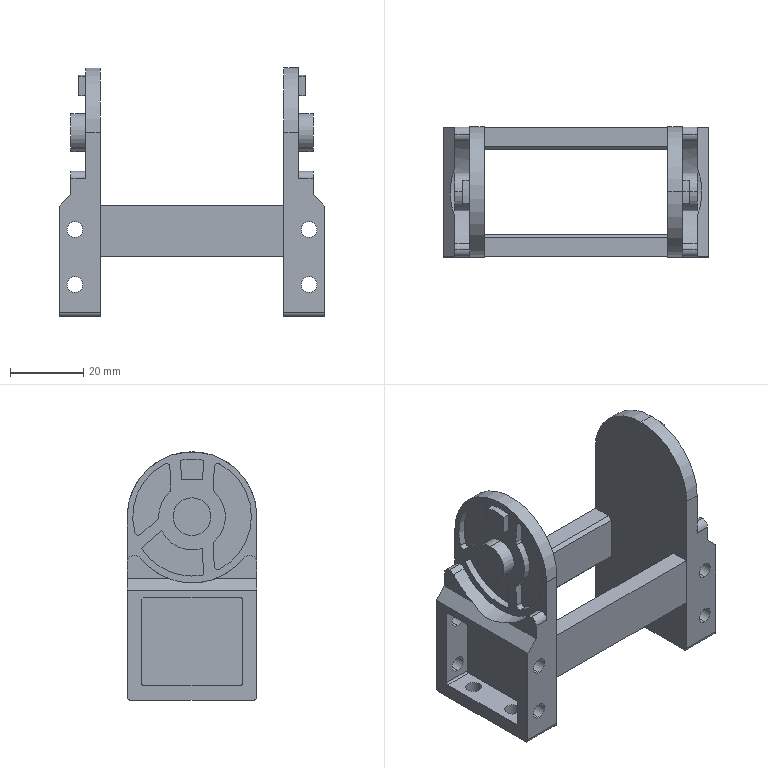Part | SolidWorks | features BaseBody 1 | 1 solid | 160 faces | box 72.4 x 35.35 x 67.664 mm | volume 31284 mm3 | cylinder 88 | plane 72 | commonest cylinder face diameters 4.3 x24 2 x21 4 x8 1 x6 10.3 x4 18.2 x4